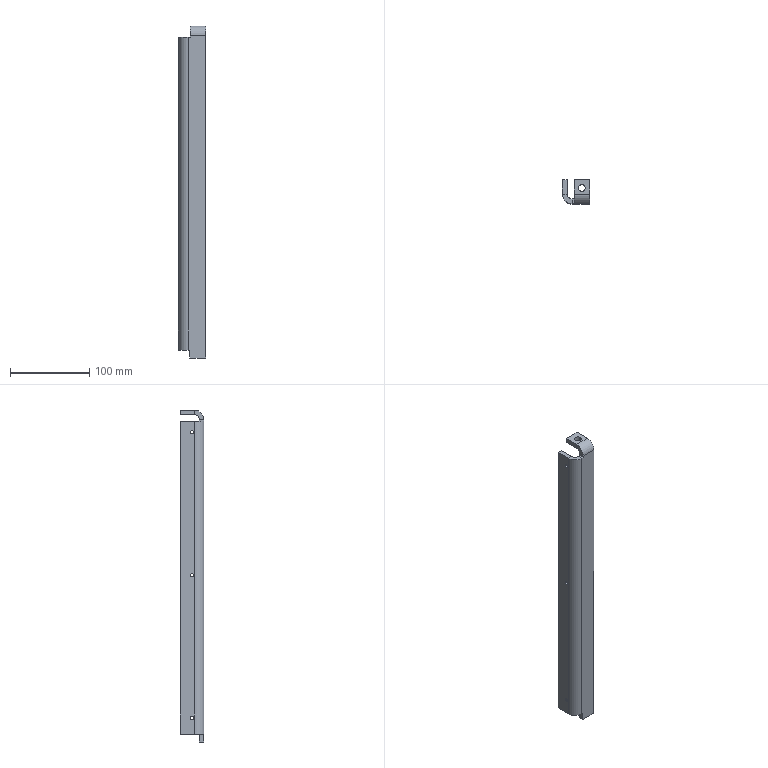Part | SolidWorks | features ICE 3, EdgeFlange 1, FlatPattern 1, SMBaseFlange 1, SheetMetal 1 | 1 solid | 34 faces | box 34 x 30 x 418 mm | volume 132505 mm3 | plane 22 | cylinder 12 | commonest cylinder face diameters 4 x6 8.5 x2 12 x2 24 x2
STEP:
#1=CARTESIAN_POINT('',(6.,15.,28.));
#2=VERTEX_POINT('',#1);
#3=CARTESIAN_POINT('',(6.,15.,32.));
#4=VERTEX_POINT('',#3);
#5=CARTESIAN_POINT('',(6.,15.,30.));
#6=DIRECTION('',(-1.,0.,0.));
#7=DIRECTION('',(0.,0.,1.));
#8=AXIS2_PLACEMENT_3D('',#5,#6,#7);
#9=CIRCLE('',#8,2.);
#10=EDGE_CURVE('',#2,#4,#9,.T.);
#11=ORIENTED_EDGE('',*,*,#10,.F.);
#12=CARTESIAN_POINT('',(0.,15.,28.));
#13=VERTEX_POINT('',#12);
#14=CARTESIAN_POINT('',(14.,15.,28.));
#15=DIRECTION('',(-1.,0.,0.));
#16=VECTOR('',#15,1000.);
#17=LINE('',#14,#16);
#18=EDGE_CURVE('',#2,#13,#17,.T.);
#19=ORIENTED_EDGE('',*,*,#18,.T.);
#20=CARTESIAN_POINT('',(0.,15.,32.));
#21=VERTEX_POINT('',#20);
#22=CARTESIAN_POINT('',(0.,15.,30.));
#23=DIRECTION('',(-1.,0.,0.));
#24=DIRECTION('',(0.,0.,1.));
#25=AXIS2_PLACEMENT_3D('',#22,#23,#24);
#26=CIRCLE('',#25,2.);
#27=EDGE_CURVE('',#13,#21,#26,.T.);
#28=ORIENTED_EDGE('',*,*,#27,.T.);
#29=CARTESIAN_POINT('',(14.,15.,32.));
#30=DIRECTION('',(-1.,0.,0.));
#31=VECTOR('',#30,1000.);
#32=LINE('',#29,#31);
#33=EDGE_CURVE('',#4,#21,#32,.T.);
#34=ORIENTED_EDGE('',*,*,#33,.F.);
#35=EDGE_LOOP('',(#11,#19,#28,#34));
#36=FACE_OUTER_BOUND('',#35,.T.);
#37=CARTESIAN_POINT('',(14.,15.,30.));
#38=DIRECTION('',(-1.,0.,0.));
#39=DIRECTION('',(0.,0.,1.));
#40=AXIS2_PLACEMENT_3D('',#37,#38,#39);
#41=CYLINDRICAL_SURFACE('',#40,2.);
#42=ADVANCED_FACE('',(#36),#41,.F.);
#43=CARTESIAN_POINT('',(6.,15.,208.));
#44=VERTEX_POINT('',#43);
#45=CARTESIAN_POINT('',(6.,15.,212.));
#46=VERTEX_POINT('',#45);
#47=CARTESIAN_POINT('',(6.,15.,210.));
#48=DIRECTION('',(-1.,0.,0.));
#49=DIRECTION('',(0.,0.,1.));
#50=AXIS2_PLACEMENT_3D('',#47,#48,#49);
#51=CIRCLE('',#50,2.);
#52=EDGE_CURVE('',#44,#46,#51,.T.);
#53=ORIENTED_EDGE('',*,*,#52,.F.);
#54=CARTESIAN_POINT('',(0.,15.,208.));
#55=VERTEX_POINT('',#54);
#56=CARTESIAN_POINT('',(14.,15.,208.));
#57=DIRECTION('',(-1.,0.,0.));
#58=VECTOR('',#57,1000.);
#59=LINE('',#56,#58);
#60=EDGE_CURVE('',#44,#55,#59,.T.);
#61=ORIENTED_EDGE('',*,*,#60,.T.);
#62=CARTESIAN_POINT('',(0.,15.,212.));
#63=VERTEX_POINT('',#62);
#64=CARTESIAN_POINT('',(0.,15.,210.));
#65=DIRECTION('',(-1.,0.,0.));
#66=DIRECTION('',(0.,0.,1.));
#67=AXIS2_PLACEMENT_3D('',#64,#65,#66);
#68=CIRCLE('',#67,2.);
#69=EDGE_CURVE('',#55,#63,#68,.T.);
#70=ORIENTED_EDGE('',*,*,#69,.T.);
#71=CARTESIAN_POINT('',(14.,15.,212.));
#72=DIRECTION('',(-1.,0.,0.));
#73=VECTOR('',#72,1000.);
#74=LINE('',#71,#73);
#75=EDGE_CURVE('',#46,#63,#74,.T.);
#76=ORIENTED_EDGE('',*,*,#75,.F.);
#77=EDGE_LOOP('',(#53,#61,#70,#76));
#78=FACE_OUTER_BOUND('',#77,.T.);
#79=CARTESIAN_POINT('',(14.,15.,210.));
#80=DIRECTION('',(-1.,0.,0.));
#81=DIRECTION('',(0.,0.,1.));
#82=AXIS2_PLACEMENT_3D('',#79,#80,#81);
#83=CYLINDRICAL_SURFACE('',#82,2.);
#84=ADVANCED_FACE('',(#78),#83,.F.);
#85=CARTESIAN_POINT('',(6.,15.,388.));
#86=VERTEX_POINT('',#85);
#87=CARTESIAN_POINT('',(6.,15.,392.));
#88=VERTEX_POINT('',#87);
#89=CARTESIAN_POINT('',(6.,15.,390.));
#90=DIRECTION('',(-1.,0.,0.));
#91=DIRECTION('',(0.,0.,1.));
#92=AXIS2_PLACEMENT_3D('',#89,#90,#91);
#93=CIRCLE('',#92,2.);
#94=EDGE_CURVE('',#86,#88,#93,.T.);
#95=ORIENTED_EDGE('',*,*,#94,.F.);
#96=CARTESIAN_POINT('',(0.,15.,388.));
#97=VERTEX_POINT('',#96);
#98=CARTESIAN_POINT('',(14.,15.,388.));
#99=DIRECTION('',(-1.,0.,0.));
#100=VECTOR('',#99,1000.);
#101=LINE('',#98,#100);
#102=EDGE_CURVE('',#86,#97,#101,.T.);
#103=ORIENTED_EDGE('',*,*,#102,.T.);
#104=CARTESIAN_POINT('',(0.,15.,392.));
#105=VERTEX_POINT('',#104);
#106=CARTESIAN_POINT('',(0.,15.,390.));
#107=DIRECTION('',(-1.,0.,0.));
#108=DIRECTION('',(0.,0.,1.));
#109=AXIS2_PLACEMENT_3D('',#106,#107,#108);
#110=CIRCLE('',#109,2.);
#111=EDGE_CURVE('',#97,#105,#110,.T.);
#112=ORIENTED_EDGE('',*,*,#111,.T.);
#113=CARTESIAN_POINT('',(14.,15.,392.));
#114=DIRECTION('',(-1.,0.,0.));
#115=VECTOR('',#114,1000.);
#116=LINE('',#113,#115);
#117=EDGE_CURVE('',#88,#105,#116,.T.);
#118=ORIENTED_EDGE('',*,*,#117,.F.);
#119=EDGE_LOOP('',(#95,#103,#112,#118));
#120=FACE_OUTER_BOUND('',#119,.T.);
#121=CARTESIAN_POINT('',(14.,15.,390.));
#122=DIRECTION('',(-1.,0.,0.));
#123=DIRECTION('',(0.,0.,1.));
#124=AXIS2_PLACEMENT_3D('',#121,#122,#123);
#125=CYLINDRICAL_SURFACE('',#124,2.);
#126=ADVANCED_FACE('',(#120),#125,.F.);
#127=CARTESIAN_POINT('',(20.25,19.5,412.));
#128=VERTEX_POINT('',#127);
#129=CARTESIAN_POINT('',(28.75,19.5,412.));
#130=VERTEX_POINT('',#129);
#131=CARTESIAN_POINT('',(24.5,19.5,412.));
#132=DIRECTION('',(0.,0.,1.));
#133=DIRECTION('',(0.,-1.,0.));
#134=AXIS2_PLACEMENT_3D('',#131,#132,#133);
#135=CIRCLE('',#134,4.25);
#136=EDGE_CURVE('',#128,#130,#135,.T.);
#137=ORIENTED_EDGE('',*,*,#136,.F.);
#138=CARTESIAN_POINT('',(20.25,19.5,418.));
#139=VERTEX_POINT('',#138);
#140=CARTESIAN_POINT('',(20.25,19.5,0.));
#141=DIRECTION('',(0.,0.,1.));
#142=VECTOR('',#141,1000.);
#143=LINE('',#140,#142);
#144=EDGE_CURVE('',#128,#139,#143,.T.);
#145=ORIENTED_EDGE('',*,*,#144,.T.);
#146=CARTESIAN_POINT('',(28.75,19.5,418.));
#147=VERTEX_POINT('',#146);
#148=CARTESIAN_POINT('',(24.5,19.5,418.));
#149=DIRECTION('',(0.,0.,1.));
#150=DIRECTION('',(1.,0.,0.));
#151=AXIS2_PLACEMENT_3D('',#148,#149,#150);
#152=CIRCLE('',#151,4.25);
#153=EDGE_CURVE('',#139,#147,#152,.T.);
#154=ORIENTED_EDGE('',*,*,#153,.T.);
#155=CARTESIAN_POINT('',(28.75,19.5,0.));
#156=DIRECTION('',(0.,0.,1.));
#157=VECTOR('',#156,1000.);
#158=LINE('',#155,#157);
#159=EDGE_CURVE('',#130,#147,#158,.T.);
#160=ORIENTED_EDGE('',*,*,#159,.F.);
#161=EDGE_LOOP('',(#137,#145,#154,#160));
#162=FACE_OUTER_BOUND('',#161,.T.);
#163=CARTESIAN_POINT('',(24.5,19.5,0.));
#164=DIRECTION('',(0.,0.,1.));
#165=DIRECTION('',(1.,0.,0.));
#166=AXIS2_PLACEMENT_3D('',#163,#164,#165);
#167=CYLINDRICAL_SURFACE('',#166,4.25);
#168=ADVANCED_FACE('',(#162),#167,.F.);
#169=CARTESIAN_POINT('',(6.,12.,10.));
#170=VERTEX_POINT('',#169);
#171=CARTESIAN_POINT('',(6.,30.,10.));
#172=VERTEX_POINT('',#171);
#173=CARTESIAN_POINT('',(6.,0.,10.));
#174=DIRECTION('',(0.,1.,0.));
#175=VECTOR('',#174,1000.);
#176=LINE('',#173,#175);
#177=EDGE_CURVE('',#170,#172,#176,.T.);
#178=ORIENTED_EDGE('',*,*,#177,.F.);
#179=CARTESIAN_POINT('',(0.,12.,10.));
#180=VERTEX_POINT('',#179);
#181=CARTESIAN_POINT('',(6.,12.,10.));
#182=DIRECTION('',(-1.,0.,0.));
#183=VECTOR('',#182,1000.);
#184=LINE('',#181,#183);
#185=EDGE_CURVE('',#170,#180,#184,.T.);
#186=ORIENTED_EDGE('',*,*,#185,.T.);
#187=CARTESIAN_POINT('',(0.,30.,10.));
#188=VERTEX_POINT('',#187);
#189=CARTESIAN_POINT('',(0.,0.,10.));
#190=DIRECTION('',(0.,1.,0.));
#191=VECTOR('',#190,1000.);
#192=LINE('',#189,#191);
#193=EDGE_CURVE('',#180,#188,#192,.T.);
#194=ORIENTED_EDGE('',*,*,#193,.T.);
#195=CARTESIAN_POINT('',(14.,30.,10.));
#196=DIRECTION('',(-1.,0.,0.));
#197=VECTOR('',#196,1000.);
#198=LINE('',#195,#197);
#199=EDGE_CURVE('',#172,#188,#198,.T.);
#200=ORIENTED_EDGE('',*,*,#199,.F.);
#201=EDGE_LOOP('',(#178,#186,#194,#200));
#202=FACE_OUTER_BOUND('',#201,.T.);
#203=CARTESIAN_POINT('',(14.,0.,10.));
#204=DIRECTION('',(0.,0.,1.));
#205=DIRECTION('',(0.,-1.,0.));
#206=AXIS2_PLACEMENT_3D('',#203,#204,#205);
#207=PLANE('',#206);
#208=ADVANCED_FACE('',(#202),#207,.F.);
#209=CARTESIAN_POINT('',(14.,0.,10.));
#210=VERTEX_POINT('',#209);
#211=CARTESIAN_POINT('',(12.,0.,10.));
#212=VERTEX_POINT('',#211);
#213=CARTESIAN_POINT('',(14.,0.,10.));
#214=DIRECTION('',(-1.,0.,0.));
#215=VECTOR('',#214,1000.);
#216=LINE('',#213,#215);
#217=EDGE_CURVE('',#210,#212,#216,.T.);
#218=ORIENTED_EDGE('',*,*,#217,.T.);
#219=CARTESIAN_POINT('',(12.,6.,10.));
#220=VERTEX_POINT('',#219);
#221=CARTESIAN_POINT('',(12.,0.,10.));
#222=DIRECTION('',(0.,1.,0.));
#223=VECTOR('',#222,1000.);
#224=LINE('',#221,#223);
#225=EDGE_CURVE('',#212,#220,#224,.T.);
#226=ORIENTED_EDGE('',*,*,#225,.T.);
#227=CARTESIAN_POINT('',(14.,6.,10.));
#228=VERTEX_POINT('',#227);
#229=CARTESIAN_POINT('',(0.,6.,10.));
#230=DIRECTION('',(-1.,0.,0.));
#231=VECTOR('',#230,1000.);
#232=LINE('',#229,#231);
#233=EDGE_CURVE('',#228,#220,#232,.T.);
#234=ORIENTED_EDGE('',*,*,#233,.F.);
#235=CARTESIAN_POINT('',(14.,0.,10.));
#236=DIRECTION('',(0.,1.,0.));
#237=VECTOR('',#236,1000.);
#238=LINE('',#235,#237);
#239=EDGE_CURVE('',#210,#228,#238,.T.);
#240=ORIENTED_EDGE('',*,*,#239,.F.);
#241=EDGE_LOOP('',(#218,#226,#234,#240));
#242=FACE_OUTER_BOUND('',#241,.T.);
#243=CARTESIAN_POINT('',(14.,0.,10.));
#244=DIRECTION('',(0.,0.,1.));
#245=DIRECTION('',(0.,-1.,0.));
#246=AXIS2_PLACEMENT_3D('',#243,#244,#245);
#247=PLANE('',#246);
#248=ADVANCED_FACE('',(#242),#247,.F.);
#249=CARTESIAN_POINT('',(12.,6.,404.));
#250=VERTEX_POINT('',#249);
#251=CARTESIAN_POINT('',(15.,6.,404.));
#252=VERTEX_POINT('',#251);
#253=CARTESIAN_POINT('',(0.,6.,404.));
#254=DIRECTION('',(1.,0.,0.));
#255=VECTOR('',#254,1000.);
#256=LINE('',#253,#255);
#257=EDGE_CURVE('',#250,#252,#256,.T.);
#258=ORIENTED_EDGE('',*,*,#257,.F.);
#259=CARTESIAN_POINT('',(12.,0.,404.));
#260=VERTEX_POINT('',#259);
#261=CARTESIAN_POINT('',(12.,6.,404.));
#262=DIRECTION('',(0.,-1.,0.));
#263=VECTOR('',#262,1000.);
#264=LINE('',#261,#263);
#265=EDGE_CURVE('',#250,#260,#264,.T.);
#266=ORIENTED_EDGE('',*,*,#265,.T.);
#267=CARTESIAN_POINT('',(15.,0.,404.));
#268=VERTEX_POINT('',#267);
#269=CARTESIAN_POINT('',(0.,0.,404.));
#270=DIRECTION('',(-1.,0.,0.));
#271=VECTOR('',#270,1000.);
#272=LINE('',#269,#271);
#273=EDGE_CURVE('',#268,#260,#272,.T.);
#274=ORIENTED_EDGE('',*,*,#273,.F.);
#275=CARTESIAN_POINT('',(15.,0.,404.));
#276=DIRECTION('',(0.,1.,0.));
#277=VECTOR('',#276,1000.);
#278=LINE('',#275,#277);
#279=EDGE_CURVE('',#268,#252,#278,.T.);
#280=ORIENTED_EDGE('',*,*,#279,.T.);
#281=EDGE_LOOP('',(#258,#266,#274,#280));
#282=FACE_OUTER_BOUND('',#281,.T.);
#283=CARTESIAN_POINT('',(0.,0.,404.));
#284=DIRECTION('',(0.,0.,-1.));
#285=DIRECTION('',(-1.,0.,0.));
#286=AXIS2_PLACEMENT_3D('',#283,#284,#285);
#287=PLANE('',#286);
#288=ADVANCED_FACE('',(#282),#287,.F.);
#289=CARTESIAN_POINT('',(0.,12.,404.));
#290=VERTEX_POINT('',#289);
#291=CARTESIAN_POINT('',(0.,30.,404.));
#292=VERTEX_POINT('',#291);
#293=CARTESIAN_POINT('',(0.,0.,404.));
#294=DIRECTION('',(0.,1.,0.));
#295=VECTOR('',#294,1000.);
#296=LINE('',#293,#295);
#297=EDGE_CURVE('',#290,#292,#296,.T.);
#298=ORIENTED_EDGE('',*,*,#297,.F.);
#299=CARTESIAN_POINT('',(6.,12.,404.));
#300=VERTEX_POINT('',#299);
#301=CARTESIAN_POINT('',(0.,12.,404.));
#302=DIRECTION('',(1.,0.,0.));
#303=VECTOR('',#302,1000.);
#304=LINE('',#301,#303);
#305=EDGE_CURVE('',#290,#300,#304,.T.);
#306=ORIENTED_EDGE('',*,*,#305,.T.);
#307=CARTESIAN_POINT('',(6.,30.,404.));
#308=VERTEX_POINT('',#307);
#309=CARTESIAN_POINT('',(6.,0.,404.));
#310=DIRECTION('',(0.,-1.,0.));
#311=VECTOR('',#310,1000.);
#312=LINE('',#309,#311);
#313=EDGE_CURVE('',#308,#300,#312,.T.);
#314=ORIENTED_EDGE('',*,*,#313,.F.);
#315=CARTESIAN_POINT('',(0.,30.,404.));
#316=DIRECTION('',(-1.,0.,0.));
#317=VECTOR('',#316,1000.);
#318=LINE('',#315,#317);
#319=EDGE_CURVE('',#308,#292,#318,.T.);
#320=ORIENTED_EDGE('',*,*,#319,.T.);
#321=EDGE_LOOP('',(#298,#306,#314,#320));
#322=FACE_OUTER_BOUND('',#321,.T.);
#323=CARTESIAN_POINT('',(0.,0.,404.));
#324=DIRECTION('',(0.,0.,-1.));
#325=DIRECTION('',(-1.,0.,0.));
#326=AXIS2_PLACEMENT_3D('',#323,#324,#325);
#327=PLANE('',#326);
#328=ADVANCED_FACE('',(#322),#327,.F.);
#329=CARTESIAN_POINT('',(14.,6.,0.));
#330=VERTEX_POINT('',#329);
#331=CARTESIAN_POINT('',(14.,0.,0.));
#332=VERTEX_POINT('',#331);
#333=CARTESIAN_POINT('',(14.,0.,0.));
#334=DIRECTION('',(0.,-1.,0.));
#335=VECTOR('',#334,1000.);
#336=LINE('',#333,#335);
#337=EDGE_CURVE('',#330,#332,#336,.T.);
#338=ORIENTED_EDGE('',*,*,#337,.F.);
#339=CARTESIAN_POINT('',(34.,6.,0.));
#340=VERTEX_POINT('',#339);
#341=CARTESIAN_POINT('',(0.,6.,0.));
#342=DIRECTION('',(-1.,0.,0.));
#343=VECTOR('',#342,1000.);
#344=LINE('',#341,#343);
#345=EDGE_CURVE('',#340,#330,#344,.T.);
#346=ORIENTED_EDGE('',*,*,#345,.F.);
#347=CARTESIAN_POINT('',(34.,0.,0.));
#348=VERTEX_POINT('',#347);
#349=CARTESIAN_POINT('',(34.,6.,0.));
#350=DIRECTION('',(0.,-1.,0.));
#351=VECTOR('',#350,1000.);
#352=LINE('',#349,#351);
#353=EDGE_CURVE('',#340,#348,#352,.T.);
#354=ORIENTED_EDGE('',*,*,#353,.T.);
#355=CARTESIAN_POINT('',(0.,0.,0.));
#356=DIRECTION('',(-1.,0.,0.));
#357=VECTOR('',#356,1000.);
#358=LINE('',#355,#357);
#359=EDGE_CURVE('',#348,#332,#358,.T.);
#360=ORIENTED_EDGE('',*,*,#359,.T.);
#361=EDGE_LOOP('',(#338,#346,#354,#360));
#362=FACE_OUTER_BOUND('',#361,.T.);
#363=CARTESIAN_POINT('',(6.,12.,0.));
#364=DIRECTION('',(0.,0.,-1.));
#365=DIRECTION('',(-1.,0.,0.));
#366=AXIS2_PLACEMENT_3D('',#363,#364,#365);
#367=PLANE('',#366);
#368=ADVANCED_FACE('',(#362),#367,.T.);
#369=CARTESIAN_POINT('',(6.,15.,30.));
#370=DIRECTION('',(-1.,0.,0.));
#371=DIRECTION('',(0.,0.,1.));
#372=AXIS2_PLACEMENT_3D('',#369,#370,#371);
#373=CIRCLE('',#372,2.);
#374=EDGE_CURVE('',#4,#2,#373,.T.);
#375=ORIENTED_EDGE('',*,*,#374,.T.);
#376=ORIENTED_EDGE('',*,*,#10,.T.);
#377=EDGE_LOOP('',(#375,#376));
#378=FACE_BOUND('',#377,.T.);
#379=CARTESIAN_POINT('',(6.,15.,210.));
#380=DIRECTION('',(-1.,0.,0.));
#381=DIRECTION('',(0.,0.,1.));
#382=AXIS2_PLACEMENT_3D('',#379,#380,#381);
#383=CIRCLE('',#382,2.);
#384=EDGE_CURVE('',#46,#44,#383,.T.);
#385=ORIENTED_EDGE('',*,*,#384,.T.);
#386=ORIENTED_EDGE('',*,*,#52,.T.);
#387=EDGE_LOOP('',(#385,#386));
#388=FACE_BOUND('',#387,.T.);
#389=CARTESIAN_POINT('',(6.,15.,390.));
#390=DIRECTION('',(-1.,0.,0.));
#391=DIRECTION('',(0.,0.,1.));
#392=AXIS2_PLACEMENT_3D('',#389,#390,#391);
#393=CIRCLE('',#392,2.);
#394=EDGE_CURVE('',#88,#86,#393,.T.);
#395=ORIENTED_EDGE('',*,*,#394,.T.);
#396=ORIENTED_EDGE('',*,*,#94,.T.);
#397=EDGE_LOOP('',(#395,#396));
#398=FACE_BOUND('',#397,.T.);
#399=CARTESIAN_POINT('',(6.,12.,406.));
#400=DIRECTION('',(0.,0.,-1.));
#401=VECTOR('',#400,1000.);
#402=LINE('',#399,#401);
#403=EDGE_CURVE('',#300,#170,#402,.T.);
#404=ORIENTED_EDGE('',*,*,#403,.T.);
#405=ORIENTED_EDGE('',*,*,#177,.T.);
#406=CARTESIAN_POINT('',(6.,30.,406.));
#407=DIRECTION('',(0.,0.,-1.));
#408=VECTOR('',#407,1000.);
#409=LINE('',#406,#408);
#410=EDGE_CURVE('',#308,#172,#409,.T.);
#411=ORIENTED_EDGE('',*,*,#410,.F.);
#412=ORIENTED_EDGE('',*,*,#313,.T.);
#413=EDGE_LOOP('',(#404,#405,#411,#412));
#414=FACE_OUTER_BOUND('',#413,.T.);
#415=CARTESIAN_POINT('',(6.,0.,406.));
#416=DIRECTION('',(-1.,0.,0.));
#417=DIRECTION('',(0.,0.,1.));
#418=AXIS2_PLACEMENT_3D('',#415,#416,#417);
#419=PLANE('',#418);
#420=ADVANCED_FACE('',(#378,#388,#398,#414),#419,.F.);
#421=ORIENTED_EDGE('',*,*,#199,.T.);
#422=CARTESIAN_POINT('',(0.,30.,406.));
#423=DIRECTION('',(0.,0.,-1.));
#424=VECTOR('',#423,1000.);
#425=LINE('',#422,#424);
#426=EDGE_CURVE('',#292,#188,#425,.T.);
#427=ORIENTED_EDGE('',*,*,#426,.F.);
#428=ORIENTED_EDGE('',*,*,#319,.F.);
#429=ORIENTED_EDGE('',*,*,#410,.T.);
#430=EDGE_LOOP('',(#421,#427,#428,#429));
#431=FACE_OUTER_BOUND('',#430,.T.);
#432=CARTESIAN_POINT('',(0.,30.,406.));
#433=DIRECTION('',(0.,1.,0.));
#434=DIRECTION('',(0.,0.,1.));
#435=AXIS2_PLACEMENT_3D('',#432,#433,#434);
#436=PLANE('',#435);
#437=ADVANCED_FACE('',(#431),#436,.T.);
#438=ORIENTED_EDGE('',*,*,#193,.F.);
#439=CARTESIAN_POINT('',(0.,12.,406.));
#440=DIRECTION('',(0.,0.,-1.));
#441=VECTOR('',#440,1000.);
#442=LINE('',#439,#441);
#443=EDGE_CURVE('',#290,#180,#442,.T.);
#444=ORIENTED_EDGE('',*,*,#443,.F.);
#445=ORIENTED_EDGE('',*,*,#297,.T.);
#446=ORIENTED_EDGE('',*,*,#426,.T.);
#447=EDGE_LOOP('',(#438,#444,#445,#446));
#448=FACE_OUTER_BOUND('',#447,.T.);
#449=CARTESIAN_POINT('',(0.,15.,30.));
#450=DIRECTION('',(-1.,0.,0.));
#451=DIRECTION('',(0.,0.,1.));
#452=AXIS2_PLACEMENT_3D('',#449,#450,#451);
#453=CIRCLE('',#452,2.);
#454=EDGE_CURVE('',#21,#13,#453,.T.);
#455=ORIENTED_EDGE('',*,*,#454,.F.);
#456=ORIENTED_EDGE('',*,*,#27,.F.);
#457=EDGE_LOOP('',(#455,#456));
#458=FACE_BOUND('',#457,.T.);
#459=CARTESIAN_POINT('',(0.,15.,210.));
#460=DIRECTION('',(-1.,0.,0.));
#461=DIRECTION('',(0.,0.,1.));
#462=AXIS2_PLACEMENT_3D('',#459,#460,#461);
#463=CIRCLE('',#462,2.);
#464=EDGE_CURVE('',#63,#55,#463,.T.);
#465=ORIENTED_EDGE('',*,*,#464,.F.);
#466=ORIENTED_EDGE('',*,*,#69,.F.);
#467=EDGE_LOOP('',(#465,#466));
#468=FACE_BOUND('',#467,.T.);
#469=CARTESIAN_POINT('',(0.,15.,390.));
#470=DIRECTION('',(-1.,0.,0.));
#471=DIRECTION('',(0.,0.,1.));
#472=AXIS2_PLACEMENT_3D('',#469,#470,#471);
#473=CIRCLE('',#472,2.);
#474=EDGE_CURVE('',#105,#97,#473,.T.);
#475=ORIENTED_EDGE('',*,*,#474,.F.);
#476=ORIENTED_EDGE('',*,*,#111,.F.);
#477=EDGE_LOOP('',(#475,#476));
#478=FACE_BOUND('',#477,.T.);
#479=CARTESIAN_POINT('',(0.,0.,406.));
#480=DIRECTION('',(-1.,0.,0.));
#481=DIRECTION('',(0.,0.,1.));
#482=AXIS2_PLACEMENT_3D('',#479,#480,#481);
#483=PLANE('',#482);
#484=ADVANCED_FACE('',(#448,#458,#468,#478),#483,.T.);
#485=CARTESIAN_POINT('',(12.,12.,10.));
#486=DIRECTION('',(0.,0.,-1.));
#487=DIRECTION('',(0.,-1.,0.));
#488=AXIS2_PLACEMENT_3D('',#485,#486,#487);
#489=CIRCLE('',#488,12.);
#490=EDGE_CURVE('',#212,#180,#489,.T.);
#491=ORIENTED_EDGE('',*,*,#490,.F.);
#492=CARTESIAN_POINT('',(12.,0.,406.));
#493=DIRECTION('',(0.,0.,-1.));
#494=VECTOR('',#493,1000.);
#495=LINE('',#492,#494);
#496=EDGE_CURVE('',#260,#212,#495,.T.);
#497=ORIENTED_EDGE('',*,*,#496,.F.);
#498=CARTESIAN_POINT('',(12.,12.,404.));
#499=DIRECTION('',(0.,0.,1.));
#500=DIRECTION('',(-1.,0.,0.));
#501=AXIS2_PLACEMENT_3D('',#498,#499,#500);
#502=CIRCLE('',#501,12.);
#503=EDGE_CURVE('',#290,#260,#502,.T.);
#504=ORIENTED_EDGE('',*,*,#503,.F.);
#505=ORIENTED_EDGE('',*,*,#443,.T.);
#506=EDGE_LOOP('',(#491,#497,#504,#505));
#507=FACE_OUTER_BOUND('',#506,.T.);
#508=CARTESIAN_POINT('',(12.,12.,406.));
#509=DIRECTION('',(0.,0.,-1.));
#510=DIRECTION('',(-1.,0.,0.));
#511=AXIS2_PLACEMENT_3D('',#508,#509,#510);
#512=CYLINDRICAL_SURFACE('',#511,12.);
#513=ADVANCED_FACE('',(#507),#512,.T.);
#514=ORIENTED_EDGE('',*,*,#217,.F.);
#515=CARTESIAN_POINT('',(14.,0.,0.));
#516=DIRECTION('',(0.,0.,1.));
#517=VECTOR('',#516,1000.);
#518=LINE('',#515,#517);
#519=EDGE_CURVE('',#332,#210,#518,.T.);
#520=ORIENTED_EDGE('',*,*,#519,.F.);
#521=ORIENTED_EDGE('',*,*,#359,.F.);
#522=CARTESIAN_POINT('',(34.,0.,406.));
#523=VERTEX_POINT('',#522);
#524=CARTESIAN_POINT('',(34.,0.,406.));
#525=DIRECTION('',(0.,0.,-1.));
#526=VECTOR('',#525,1000.);
#527=LINE('',#524,#526);
#528=EDGE_CURVE('',#523,#348,#527,.T.);
#529=ORIENTED_EDGE('',*,*,#528,.F.);
#530=CARTESIAN_POINT('',(15.,0.,406.));
#531=VERTEX_POINT('',#530);
#532=CARTESIAN_POINT('',(0.,0.,406.));
#533=DIRECTION('',(-1.,0.,0.));
#534=VECTOR('',#533,1000.);
#535=LINE('',#532,#534);
#536=EDGE_CURVE('',#523,#531,#535,.T.);
#537=ORIENTED_EDGE('',*,*,#536,.T.);
#538=CARTESIAN_POINT('',(15.,0.,406.));
#539=DIRECTION('',(0.,0.,-1.));
#540=VECTOR('',#539,1000.);
#541=LINE('',#538,#540);
#542=EDGE_CURVE('',#531,#268,#541,.T.);
#543=ORIENTED_EDGE('',*,*,#542,.T.);
#544=ORIENTED_EDGE('',*,*,#273,.T.);
#545=ORIENTED_EDGE('',*,*,#496,.T.);
#546=EDGE_LOOP('',(#514,#520,#521,#529,#537,#543,#544,#545));
#547=FACE_OUTER_BOUND('',#546,.T.);
#548=CARTESIAN_POINT('',(0.,0.,406.));
#549=DIRECTION('',(0.,-1.,0.));
#550=DIRECTION('',(0.,0.,-1.));
#551=AXIS2_PLACEMENT_3D('',#548,#549,#550);
#552=PLANE('',#551);
#553=ADVANCED_FACE('',(#547),#552,.T.);
#554=ORIENTED_EDGE('',*,*,#353,.F.);
#555=CARTESIAN_POINT('',(34.,6.,406.));
#556=VERTEX_POINT('',#555);
#557=CARTESIAN_POINT('',(34.,6.,406.));
#558=DIRECTION('',(0.,0.,-1.));
#559=VECTOR('',#558,1000.);
#560=LINE('',#557,#559);
#561=EDGE_CURVE('',#556,#340,#560,.T.);
#562=ORIENTED_EDGE('',*,*,#561,.F.);
#563=CARTESIAN_POINT('',(34.,6.,406.));
#564=DIRECTION('',(0.,-1.,0.));
#565=VECTOR('',#564,1000.);
#566=LINE('',#563,#565);
#567=EDGE_CURVE('',#556,#523,#566,.T.);
#568=ORIENTED_EDGE('',*,*,#567,.T.);
#569=ORIENTED_EDGE('',*,*,#528,.T.);
#570=EDGE_LOOP('',(#554,#562,#568,#569));
#571=FACE_OUTER_BOUND('',#570,.T.);
#572=CARTESIAN_POINT('',(34.,6.,406.));
#573=DIRECTION('',(1.,0.,0.));
#574=DIRECTION('',(0.,0.,-1.));
#575=AXIS2_PLACEMENT_3D('',#572,#573,#574);
#576=PLANE('',#575);
#577=ADVANCED_FACE('',(#571),#576,.T.);
#578=CARTESIAN_POINT('',(14.,6.,406.));
#579=DIRECTION('',(0.,0.,1.));
#580=VECTOR('',#579,1000.);
#581=LINE('',#578,#580);
#582=EDGE_CURVE('',#330,#228,#581,.T.);
#583=ORIENTED_EDGE('',*,*,#582,.T.);
#584=ORIENTED_EDGE('',*,*,#233,.T.);
#585=CARTESIAN_POINT('',(12.,6.,406.));
#586=DIRECTION('',(0.,0.,-1.));
#587=VECTOR('',#586,1000.);
#588=LINE('',#585,#587);
#589=EDGE_CURVE('',#250,#220,#588,.T.);
#590=ORIENTED_EDGE('',*,*,#589,.F.);
#591=ORIENTED_EDGE('',*,*,#257,.T.);
#592=CARTESIAN_POINT('',(15.,6.,406.));
#593=VERTEX_POINT('',#592);
#594=CARTESIAN_POINT('',(15.,6.,406.));
#595=DIRECTION('',(0.,0.,1.));
#596=VECTOR('',#595,1000.);
#597=LINE('',#594,#596);
#598=EDGE_CURVE('',#252,#593,#597,.T.);
#599=ORIENTED_EDGE('',*,*,#598,.T.);
#600=CARTESIAN_POINT('',(0.,6.,406.));
#601=DIRECTION('',(-1.,0.,0.));
#602=VECTOR('',#601,1000.);
#603=LINE('',#600,#602);
#604=EDGE_CURVE('',#556,#593,#603,.T.);
#605=ORIENTED_EDGE('',*,*,#604,.F.);
#606=ORIENTED_EDGE('',*,*,#561,.T.);
#607=ORIENTED_EDGE('',*,*,#345,.T.);
#608=EDGE_LOOP('',(#583,#584,#590,#591,#599,#605,#606,#607));
#609=FACE_OUTER_BOUND('',#608,.T.);
#610=CARTESIAN_POINT('',(0.,6.,406.));
#611=DIRECTION('',(0.,-1.,0.));
#612=DIRECTION('',(0.,0.,-1.));
#613=AXIS2_PLACEMENT_3D('',#610,#611,#612);
#614=PLANE('',#613);
#615=ADVANCED_FACE('',(#609),#614,.F.);
#616=ORIENTED_EDGE('',*,*,#589,.T.);
#617=CARTESIAN_POINT('',(12.,12.,10.));
#618=DIRECTION('',(0.,0.,-1.));
#619=DIRECTION('',(0.,-1.,0.));
#620=AXIS2_PLACEMENT_3D('',#617,#618,#619);
#621=CIRCLE('',#620,6.);
#622=EDGE_CURVE('',#220,#170,#621,.T.);
#623=ORIENTED_EDGE('',*,*,#622,.T.);
#624=ORIENTED_EDGE('',*,*,#403,.F.);
#625=CARTESIAN_POINT('',(12.,12.,404.));
#626=DIRECTION('',(0.,0.,1.));
#627=DIRECTION('',(-1.,0.,0.));
#628=AXIS2_PLACEMENT_3D('',#625,#626,#627);
#629=CIRCLE('',#628,6.);
#630=EDGE_CURVE('',#300,#250,#629,.T.);
#631=ORIENTED_EDGE('',*,*,#630,.T.);
#632=EDGE_LOOP('',(#616,#623,#624,#631));
#633=FACE_OUTER_BOUND('',#632,.T.);
#634=CARTESIAN_POINT('',(12.,12.,406.));
#635=DIRECTION('',(0.,0.,-1.));
#636=DIRECTION('',(-1.,0.,0.));
#637=AXIS2_PLACEMENT_3D('',#634,#635,#636);
#638=CYLINDRICAL_SURFACE('',#637,6.);
#639=ADVANCED_FACE('',(#633),#638,.F.);
#640=ORIENTED_EDGE('',*,*,#265,.F.);
#641=ORIENTED_EDGE('',*,*,#630,.F.);
#642=ORIENTED_EDGE('',*,*,#305,.F.);
#643=ORIENTED_EDGE('',*,*,#503,.T.);
#644=EDGE_LOOP('',(#640,#641,#642,#643));
#645=FACE_OUTER_BOUND('',#644,.T.);
#646=CARTESIAN_POINT('',(0.,0.,404.));
#647=DIRECTION('',(0.,0.,-1.));
#648=DIRECTION('',(-1.,0.,0.));
#649=AXIS2_PLACEMENT_3D('',#646,#647,#648);
#650=PLANE('',#649);
#651=ADVANCED_FACE('',(#645),#650,.F.);
#652=ORIENTED_EDGE('',*,*,#279,.F.);
#653=ORIENTED_EDGE('',*,*,#542,.F.);
#654=CARTESIAN_POINT('',(15.,0.,406.));
#655=DIRECTION('',(0.,1.,0.));
#656=VECTOR('',#655,1000.);
#657=LINE('',#654,#656);
#658=EDGE_CURVE('',#531,#593,#657,.T.);
#659=ORIENTED_EDGE('',*,*,#658,.T.);
#660=ORIENTED_EDGE('',*,*,#598,.F.);
#661=EDGE_LOOP('',(#652,#653,#659,#660));
#662=FACE_OUTER_BOUND('',#661,.T.);
#663=CARTESIAN_POINT('',(15.,0.,406.));
#664=DIRECTION('',(1.,0.,0.));
#665=DIRECTION('',(0.,0.,-1.));
#666=AXIS2_PLACEMENT_3D('',#663,#664,#665);
#667=PLANE('',#666);
#668=ADVANCED_FACE('',(#662),#667,.F.);
#669=CARTESIAN_POINT('',(15.,12.,412.));
#670=VERTEX_POINT('',#669);
#671=CARTESIAN_POINT('',(15.,12.,418.));
#672=VERTEX_POINT('',#671);
#673=CARTESIAN_POINT('',(15.,12.,418.));
#674=DIRECTION('',(0.,0.,1.));
#675=VECTOR('',#674,1000.);
#676=LINE('',#673,#675);
#677=EDGE_CURVE('',#670,#672,#676,.T.);
#678=ORIENTED_EDGE('',*,*,#677,.F.);
#679=CARTESIAN_POINT('',(15.,12.,406.));
#680=DIRECTION('',(-1.,0.,0.));
#681=DIRECTION('',(0.,0.,-1.));
#682=AXIS2_PLACEMENT_3D('',#679,#680,#681);
#683=CIRCLE('',#682,6.);
#684=EDGE_CURVE('',#593,#670,#683,.T.);
#685=ORIENTED_EDGE('',*,*,#684,.F.);
#686=ORIENTED_EDGE('',*,*,#658,.F.);
#687=CARTESIAN_POINT('',(15.,12.,406.));
#688=DIRECTION('',(-1.,0.,0.));
#689=DIRECTION('',(0.,0.,-1.));
#690=AXIS2_PLACEMENT_3D('',#687,#688,#689);
#691=CIRCLE('',#690,12.);
#692=EDGE_CURVE('',#531,#672,#691,.T.);
#693=ORIENTED_EDGE('',*,*,#692,.T.);
#694=EDGE_LOOP('',(#678,#685,#686,#693));
#695=FACE_OUTER_BOUND('',#694,.T.);
#696=CARTESIAN_POINT('',(15.,12.,406.));
#697=DIRECTION('',(-1.,0.,0.));
#698=DIRECTION('',(0.,0.,1.));
#699=AXIS2_PLACEMENT_3D('',#696,#697,#698);
#700=PLANE('',#699);
#701=ADVANCED_FACE('',(#695),#700,.T.);
#702=CARTESIAN_POINT('',(34.,12.,412.));
#703=VERTEX_POINT('',#702);
#704=CARTESIAN_POINT('',(34.,12.,406.));
#705=DIRECTION('',(1.,0.,0.));
#706=DIRECTION('',(0.,0.,-1.));
#707=AXIS2_PLACEMENT_3D('',#704,#705,#706);
#708=CIRCLE('',#707,6.);
#709=EDGE_CURVE('',#703,#556,#708,.T.);
#710=ORIENTED_EDGE('',*,*,#709,.F.);
#711=CARTESIAN_POINT('',(34.,12.,418.));
#712=VERTEX_POINT('',#711);
#713=CARTESIAN_POINT('',(34.,12.,412.));
#714=DIRECTION('',(0.,0.,1.));
#715=VECTOR('',#714,1000.);
#716=LINE('',#713,#715);
#717=EDGE_CURVE('',#703,#712,#716,.T.);
#718=ORIENTED_EDGE('',*,*,#717,.T.);
#719=CARTESIAN_POINT('',(34.,12.,406.));
#720=DIRECTION('',(1.,0.,0.));
#721=DIRECTION('',(0.,0.,-1.));
#722=AXIS2_PLACEMENT_3D('',#719,#720,#721);
#723=CIRCLE('',#722,12.);
#724=EDGE_CURVE('',#712,#523,#723,.T.);
#725=ORIENTED_EDGE('',*,*,#724,.T.);
#726=ORIENTED_EDGE('',*,*,#567,.F.);
#727=EDGE_LOOP('',(#710,#718,#725,#726));
#728=FACE_OUTER_BOUND('',#727,.T.);
#729=CARTESIAN_POINT('',(34.,12.,406.));
#730=DIRECTION('',(-1.,0.,0.));
#731=DIRECTION('',(0.,0.,1.));
#732=AXIS2_PLACEMENT_3D('',#729,#730,#731);
#733=PLANE('',#732);
#734=ADVANCED_FACE('',(#728),#733,.F.);
#735=ORIENTED_EDGE('',*,*,#536,.F.);
#736=ORIENTED_EDGE('',*,*,#724,.F.);
#737=CARTESIAN_POINT('',(0.,12.,418.));
#738=DIRECTION('',(1.,0.,0.));
#739=VECTOR('',#738,1000.);
#740=LINE('',#737,#739);
#741=EDGE_CURVE('',#672,#712,#740,.T.);
#742=ORIENTED_EDGE('',*,*,#741,.F.);
#743=ORIENTED_EDGE('',*,*,#692,.F.);
#744=EDGE_LOOP('',(#735,#736,#742,#743));
#745=FACE_OUTER_BOUND('',#744,.T.);
#746=CARTESIAN_POINT('',(34.,12.,406.));
#747=DIRECTION('',(1.,0.,0.));
#748=DIRECTION('',(0.,0.,1.));
#749=AXIS2_PLACEMENT_3D('',#746,#747,#748);
#750=CYLINDRICAL_SURFACE('',#749,12.);
#751=ADVANCED_FACE('',(#745),#750,.T.);
#752=ORIENTED_EDGE('',*,*,#604,.T.);
#753=ORIENTED_EDGE('',*,*,#684,.T.);
#754=CARTESIAN_POINT('',(15.,12.,412.));
#755=DIRECTION('',(1.,0.,0.));
#756=VECTOR('',#755,1000.);
#757=LINE('',#754,#756);
#758=EDGE_CURVE('',#670,#703,#757,.T.);
#759=ORIENTED_EDGE('',*,*,#758,.T.);
#760=ORIENTED_EDGE('',*,*,#709,.T.);
#761=EDGE_LOOP('',(#752,#753,#759,#760));
#762=FACE_OUTER_BOUND('',#761,.T.);
#763=CARTESIAN_POINT('',(34.,12.,406.));
#764=DIRECTION('',(1.,0.,0.));
#765=DIRECTION('',(0.,0.,1.));
#766=AXIS2_PLACEMENT_3D('',#763,#764,#765);
#767=CYLINDRICAL_SURFACE('',#766,6.);
#768=ADVANCED_FACE('',(#762),#767,.F.);
#769=CARTESIAN_POINT('',(34.,30.,418.));
#770=VERTEX_POINT('',#769);
#771=CARTESIAN_POINT('',(34.,6.,418.));
#772=DIRECTION('',(0.,-1.,0.));
#773=VECTOR('',#772,1000.);
#774=LINE('',#771,#773);
#775=EDGE_CURVE('',#770,#712,#774,.T.);
#776=ORIENTED_EDGE('',*,*,#775,.T.);
#777=ORIENTED_EDGE('',*,*,#717,.F.);
#778=CARTESIAN_POINT('',(34.,30.,412.));
#779=VERTEX_POINT('',#778);
#780=CARTESIAN_POINT('',(34.,0.,412.));
#781=DIRECTION('',(0.,-1.,0.));
#782=VECTOR('',#781,1000.);
#783=LINE('',#780,#782);
#784=EDGE_CURVE('',#779,#703,#783,.T.);
#785=ORIENTED_EDGE('',*,*,#784,.F.);
#786=CARTESIAN_POINT('',(34.,30.,418.));
#787=DIRECTION('',(0.,0.,-1.));
#788=VECTOR('',#787,1000.);
#789=LINE('',#786,#788);
#790=EDGE_CURVE('',#770,#779,#789,.T.);
#791=ORIENTED_EDGE('',*,*,#790,.F.);
#792=EDGE_LOOP('',(#776,#777,#785,#791));
#793=FACE_OUTER_BOUND('',#792,.T.);
#794=CARTESIAN_POINT('',(34.,6.,418.));
#795=DIRECTION('',(1.,0.,0.));
#796=DIRECTION('',(0.,0.,-1.));
#797=AXIS2_PLACEMENT_3D('',#794,#795,#796);
#798=PLANE('',#797);
#799=ADVANCED_FACE('',(#793),#798,.T.);
#800=CARTESIAN_POINT('',(15.,30.,412.));
#801=VERTEX_POINT('',#800);
#802=CARTESIAN_POINT('',(15.,0.,412.));
#803=DIRECTION('',(0.,1.,0.));
#804=VECTOR('',#803,1000.);
#805=LINE('',#802,#804);
#806=EDGE_CURVE('',#670,#801,#805,.T.);
#807=ORIENTED_EDGE('',*,*,#806,.F.);
#808=ORIENTED_EDGE('',*,*,#677,.T.);
#809=CARTESIAN_POINT('',(15.,30.,418.));
#810=VERTEX_POINT('',#809);
#811=CARTESIAN_POINT('',(15.,30.,418.));
#812=DIRECTION('',(0.,1.,0.));
#813=VECTOR('',#812,1000.);
#814=LINE('',#811,#813);
#815=EDGE_CURVE('',#672,#810,#814,.T.);
#816=ORIENTED_EDGE('',*,*,#815,.T.);
#817=CARTESIAN_POINT('',(15.,30.,418.));
#818=DIRECTION('',(0.,0.,-1.));
#819=VECTOR('',#818,1000.);
#820=LINE('',#817,#819);
#821=EDGE_CURVE('',#810,#801,#820,.T.);
#822=ORIENTED_EDGE('',*,*,#821,.T.);
#823=EDGE_LOOP('',(#807,#808,#816,#822));
#824=FACE_OUTER_BOUND('',#823,.T.);
#825=CARTESIAN_POINT('',(15.,30.,418.));
#826=DIRECTION('',(-1.,0.,0.));
#827=DIRECTION('',(0.,0.,1.));
#828=AXIS2_PLACEMENT_3D('',#825,#826,#827);
#829=PLANE('',#828);
#830=ADVANCED_FACE('',(#824),#829,.T.);
#831=CARTESIAN_POINT('',(24.5,19.5,418.));
#832=DIRECTION('',(0.,0.,1.));
#833=DIRECTION('',(1.,0.,0.));
#834=AXIS2_PLACEMENT_3D('',#831,#832,#833);
#835=CIRCLE('',#834,4.25);
#836=EDGE_CURVE('',#147,#139,#835,.T.);
#837=ORIENTED_EDGE('',*,*,#836,.F.);
#838=ORIENTED_EDGE('',*,*,#153,.F.);
#839=EDGE_LOOP('',(#837,#838));
#840=FACE_BOUND('',#839,.T.);
#841=ORIENTED_EDGE('',*,*,#815,.F.);
#842=ORIENTED_EDGE('',*,*,#741,.T.);
#843=ORIENTED_EDGE('',*,*,#775,.F.);
#844=CARTESIAN_POINT('',(34.,30.,418.));
#845=DIRECTION('',(1.,0.,0.));
#846=VECTOR('',#845,1000.);
#847=LINE('',#844,#846);
#848=EDGE_CURVE('',#810,#770,#847,.T.);
#849=ORIENTED_EDGE('',*,*,#848,.F.);
#850=EDGE_LOOP('',(#841,#842,#843,#849));
#851=FACE_OUTER_BOUND('',#850,.T.);
#852=CARTESIAN_POINT('',(0.,0.,418.));
#853=DIRECTION('',(0.,0.,1.));
#854=DIRECTION('',(0.,-1.,0.));
#855=AXIS2_PLACEMENT_3D('',#852,#853,#854);
#856=PLANE('',#855);
#857=ADVANCED_FACE('',(#840,#851),#856,.T.);
#858=CARTESIAN_POINT('',(24.5,19.5,412.));
#859=DIRECTION('',(0.,0.,1.));
#860=DIRECTION('',(0.,-1.,0.));
#861=AXIS2_PLACEMENT_3D('',#858,#859,#860);
#862=CIRCLE('',#861,4.25);
#863=EDGE_CURVE('',#130,#128,#862,.T.);
#864=ORIENTED_EDGE('',*,*,#863,.T.);
#865=ORIENTED_EDGE('',*,*,#136,.T.);
#866=EDGE_LOOP('',(#864,#865));
#867=FACE_BOUND('',#866,.T.);
#868=ORIENTED_EDGE('',*,*,#758,.F.);
#869=ORIENTED_EDGE('',*,*,#806,.T.);
#870=CARTESIAN_POINT('',(0.,30.,412.));
#871=DIRECTION('',(1.,0.,0.));
#872=VECTOR('',#871,1000.);
#873=LINE('',#870,#872);
#874=EDGE_CURVE('',#801,#779,#873,.T.);
#875=ORIENTED_EDGE('',*,*,#874,.T.);
#876=ORIENTED_EDGE('',*,*,#784,.T.);
#877=EDGE_LOOP('',(#868,#869,#875,#876));
#878=FACE_OUTER_BOUND('',#877,.T.);
#879=CARTESIAN_POINT('',(0.,0.,412.));
#880=DIRECTION('',(0.,0.,1.));
#881=DIRECTION('',(0.,-1.,0.));
#882=AXIS2_PLACEMENT_3D('',#879,#880,#881);
#883=PLANE('',#882);
#884=ADVANCED_FACE('',(#867,#878),#883,.F.);
#885=ORIENTED_EDGE('',*,*,#874,.F.);
#886=ORIENTED_EDGE('',*,*,#821,.F.);
#887=ORIENTED_EDGE('',*,*,#848,.T.);
#888=ORIENTED_EDGE('',*,*,#790,.T.);
#889=EDGE_LOOP('',(#885,#886,#887,#888));
#890=FACE_OUTER_BOUND('',#889,.T.);
#891=CARTESIAN_POINT('',(34.,30.,418.));
#892=DIRECTION('',(0.,1.,0.));
#893=DIRECTION('',(0.,0.,1.));
#894=AXIS2_PLACEMENT_3D('',#891,#892,#893);
#895=PLANE('',#894);
#896=ADVANCED_FACE('',(#890),#895,.T.);
#897=ORIENTED_EDGE('',*,*,#144,.F.);
#898=ORIENTED_EDGE('',*,*,#863,.F.);
#899=ORIENTED_EDGE('',*,*,#159,.T.);
#900=ORIENTED_EDGE('',*,*,#836,.T.);
#901=EDGE_LOOP('',(#897,#898,#899,#900));
#902=FACE_OUTER_BOUND('',#901,.T.);
#903=CARTESIAN_POINT('',(24.5,19.5,0.));
#904=DIRECTION('',(0.,0.,1.));
#905=DIRECTION('',(1.,0.,0.));
#906=AXIS2_PLACEMENT_3D('',#903,#904,#905);
#907=CYLINDRICAL_SURFACE('',#906,4.25);
#908=ADVANCED_FACE('',(#902),#907,.F.);
#909=ORIENTED_EDGE('',*,*,#337,.T.);
#910=ORIENTED_EDGE('',*,*,#519,.T.);
#911=ORIENTED_EDGE('',*,*,#239,.T.);
#912=ORIENTED_EDGE('',*,*,#582,.F.);
#913=EDGE_LOOP('',(#909,#910,#911,#912));
#914=FACE_OUTER_BOUND('',#913,.T.);
#915=CARTESIAN_POINT('',(14.,0.,0.));
#916=DIRECTION('',(1.,0.,0.));
#917=DIRECTION('',(0.,0.,-1.));
#918=AXIS2_PLACEMENT_3D('',#915,#916,#917);
#919=PLANE('',#918);
#920=ADVANCED_FACE('',(#914),#919,.F.);
#921=ORIENTED_EDGE('',*,*,#185,.F.);
#922=ORIENTED_EDGE('',*,*,#622,.F.);
#923=ORIENTED_EDGE('',*,*,#225,.F.);
#924=ORIENTED_EDGE('',*,*,#490,.T.);
#925=EDGE_LOOP('',(#921,#922,#923,#924));
#926=FACE_OUTER_BOUND('',#925,.T.);
#927=CARTESIAN_POINT('',(14.,0.,10.));
#928=DIRECTION('',(0.,0.,1.));
#929=DIRECTION('',(0.,-1.,0.));
#930=AXIS2_PLACEMENT_3D('',#927,#928,#929);
#931=PLANE('',#930);
#932=ADVANCED_FACE('',(#926),#931,.F.);
#933=ORIENTED_EDGE('',*,*,#102,.F.);
#934=ORIENTED_EDGE('',*,*,#394,.F.);
#935=ORIENTED_EDGE('',*,*,#117,.T.);
#936=ORIENTED_EDGE('',*,*,#474,.T.);
#937=EDGE_LOOP('',(#933,#934,#935,#936));
#938=FACE_OUTER_BOUND('',#937,.T.);
#939=CARTESIAN_POINT('',(14.,15.,390.));
#940=DIRECTION('',(-1.,0.,0.));
#941=DIRECTION('',(0.,0.,1.));
#942=AXIS2_PLACEMENT_3D('',#939,#940,#941);
#943=CYLINDRICAL_SURFACE('',#942,2.);
#944=ADVANCED_FACE('',(#938),#943,.F.);
#945=ORIENTED_EDGE('',*,*,#60,.F.);
#946=ORIENTED_EDGE('',*,*,#384,.F.);
#947=ORIENTED_EDGE('',*,*,#75,.T.);
#948=ORIENTED_EDGE('',*,*,#464,.T.);
#949=EDGE_LOOP('',(#945,#946,#947,#948));
#950=FACE_OUTER_BOUND('',#949,.T.);
#951=CARTESIAN_POINT('',(14.,15.,210.));
#952=DIRECTION('',(-1.,0.,0.));
#953=DIRECTION('',(0.,0.,1.));
#954=AXIS2_PLACEMENT_3D('',#951,#952,#953);
#955=CYLINDRICAL_SURFACE('',#954,2.);
#956=ADVANCED_FACE('',(#950),#955,.F.);
#957=ORIENTED_EDGE('',*,*,#18,.F.);
#958=ORIENTED_EDGE('',*,*,#374,.F.);
#959=ORIENTED_EDGE('',*,*,#33,.T.);
#960=ORIENTED_EDGE('',*,*,#454,.T.);
#961=EDGE_LOOP('',(#957,#958,#959,#960));
#962=FACE_OUTER_BOUND('',#961,.T.);
#963=CARTESIAN_POINT('',(14.,15.,30.));
#964=DIRECTION('',(-1.,0.,0.));
#965=DIRECTION('',(0.,0.,1.));
#966=AXIS2_PLACEMENT_3D('',#963,#964,#965);
#967=CYLINDRICAL_SURFACE('',#966,2.);
#968=ADVANCED_FACE('',(#962),#967,.F.);
#969=CLOSED_SHELL('',(#42,#84,#126,#168,#208,#248,#288,#328,#368,#420,#437,#484,#513,#553,#577,#615,#639,#651,#668,#701,#734,#751,#768,#799,#830,#857,#884,#896,#908,#920,#932,#944,#956,#968));
#970=MANIFOLD_SOLID_BREP('',#969);
#971=CARTESIAN_POINT('',(0.,0.,0.));
#972=DIRECTION('',(0.,0.,1.));
#973=DIRECTION('',(1.,0.,0.));
#974=AXIS2_PLACEMENT_3D('',#971,#972,#973);
#975=(LENGTH_UNIT()NAMED_UNIT(*)SI_UNIT(.MILLI.,.METRE.));
#976=UNCERTAINTY_MEASURE_WITH_UNIT(LENGTH_MEASURE(0.00001),#975,'','');
#977=(NAMED_UNIT(*)PLANE_ANGLE_UNIT()SI_UNIT($,.RADIAN.));
#978=(NAMED_UNIT(*)SI_UNIT($,.STERADIAN.)SOLID_ANGLE_UNIT());
#979=(GEOMETRIC_REPRESENTATION_CONTEXT(3)GLOBAL_UNCERTAINTY_ASSIGNED_CONTEXT((#976))GLOBAL_UNIT_ASSIGNED_CONTEXT((#975,#977,#978))REPRESENTATION_CONTEXT('',''));
#980=ADVANCED_BREP_SHAPE_REPRESENTATION('',(#970,#974),#979);